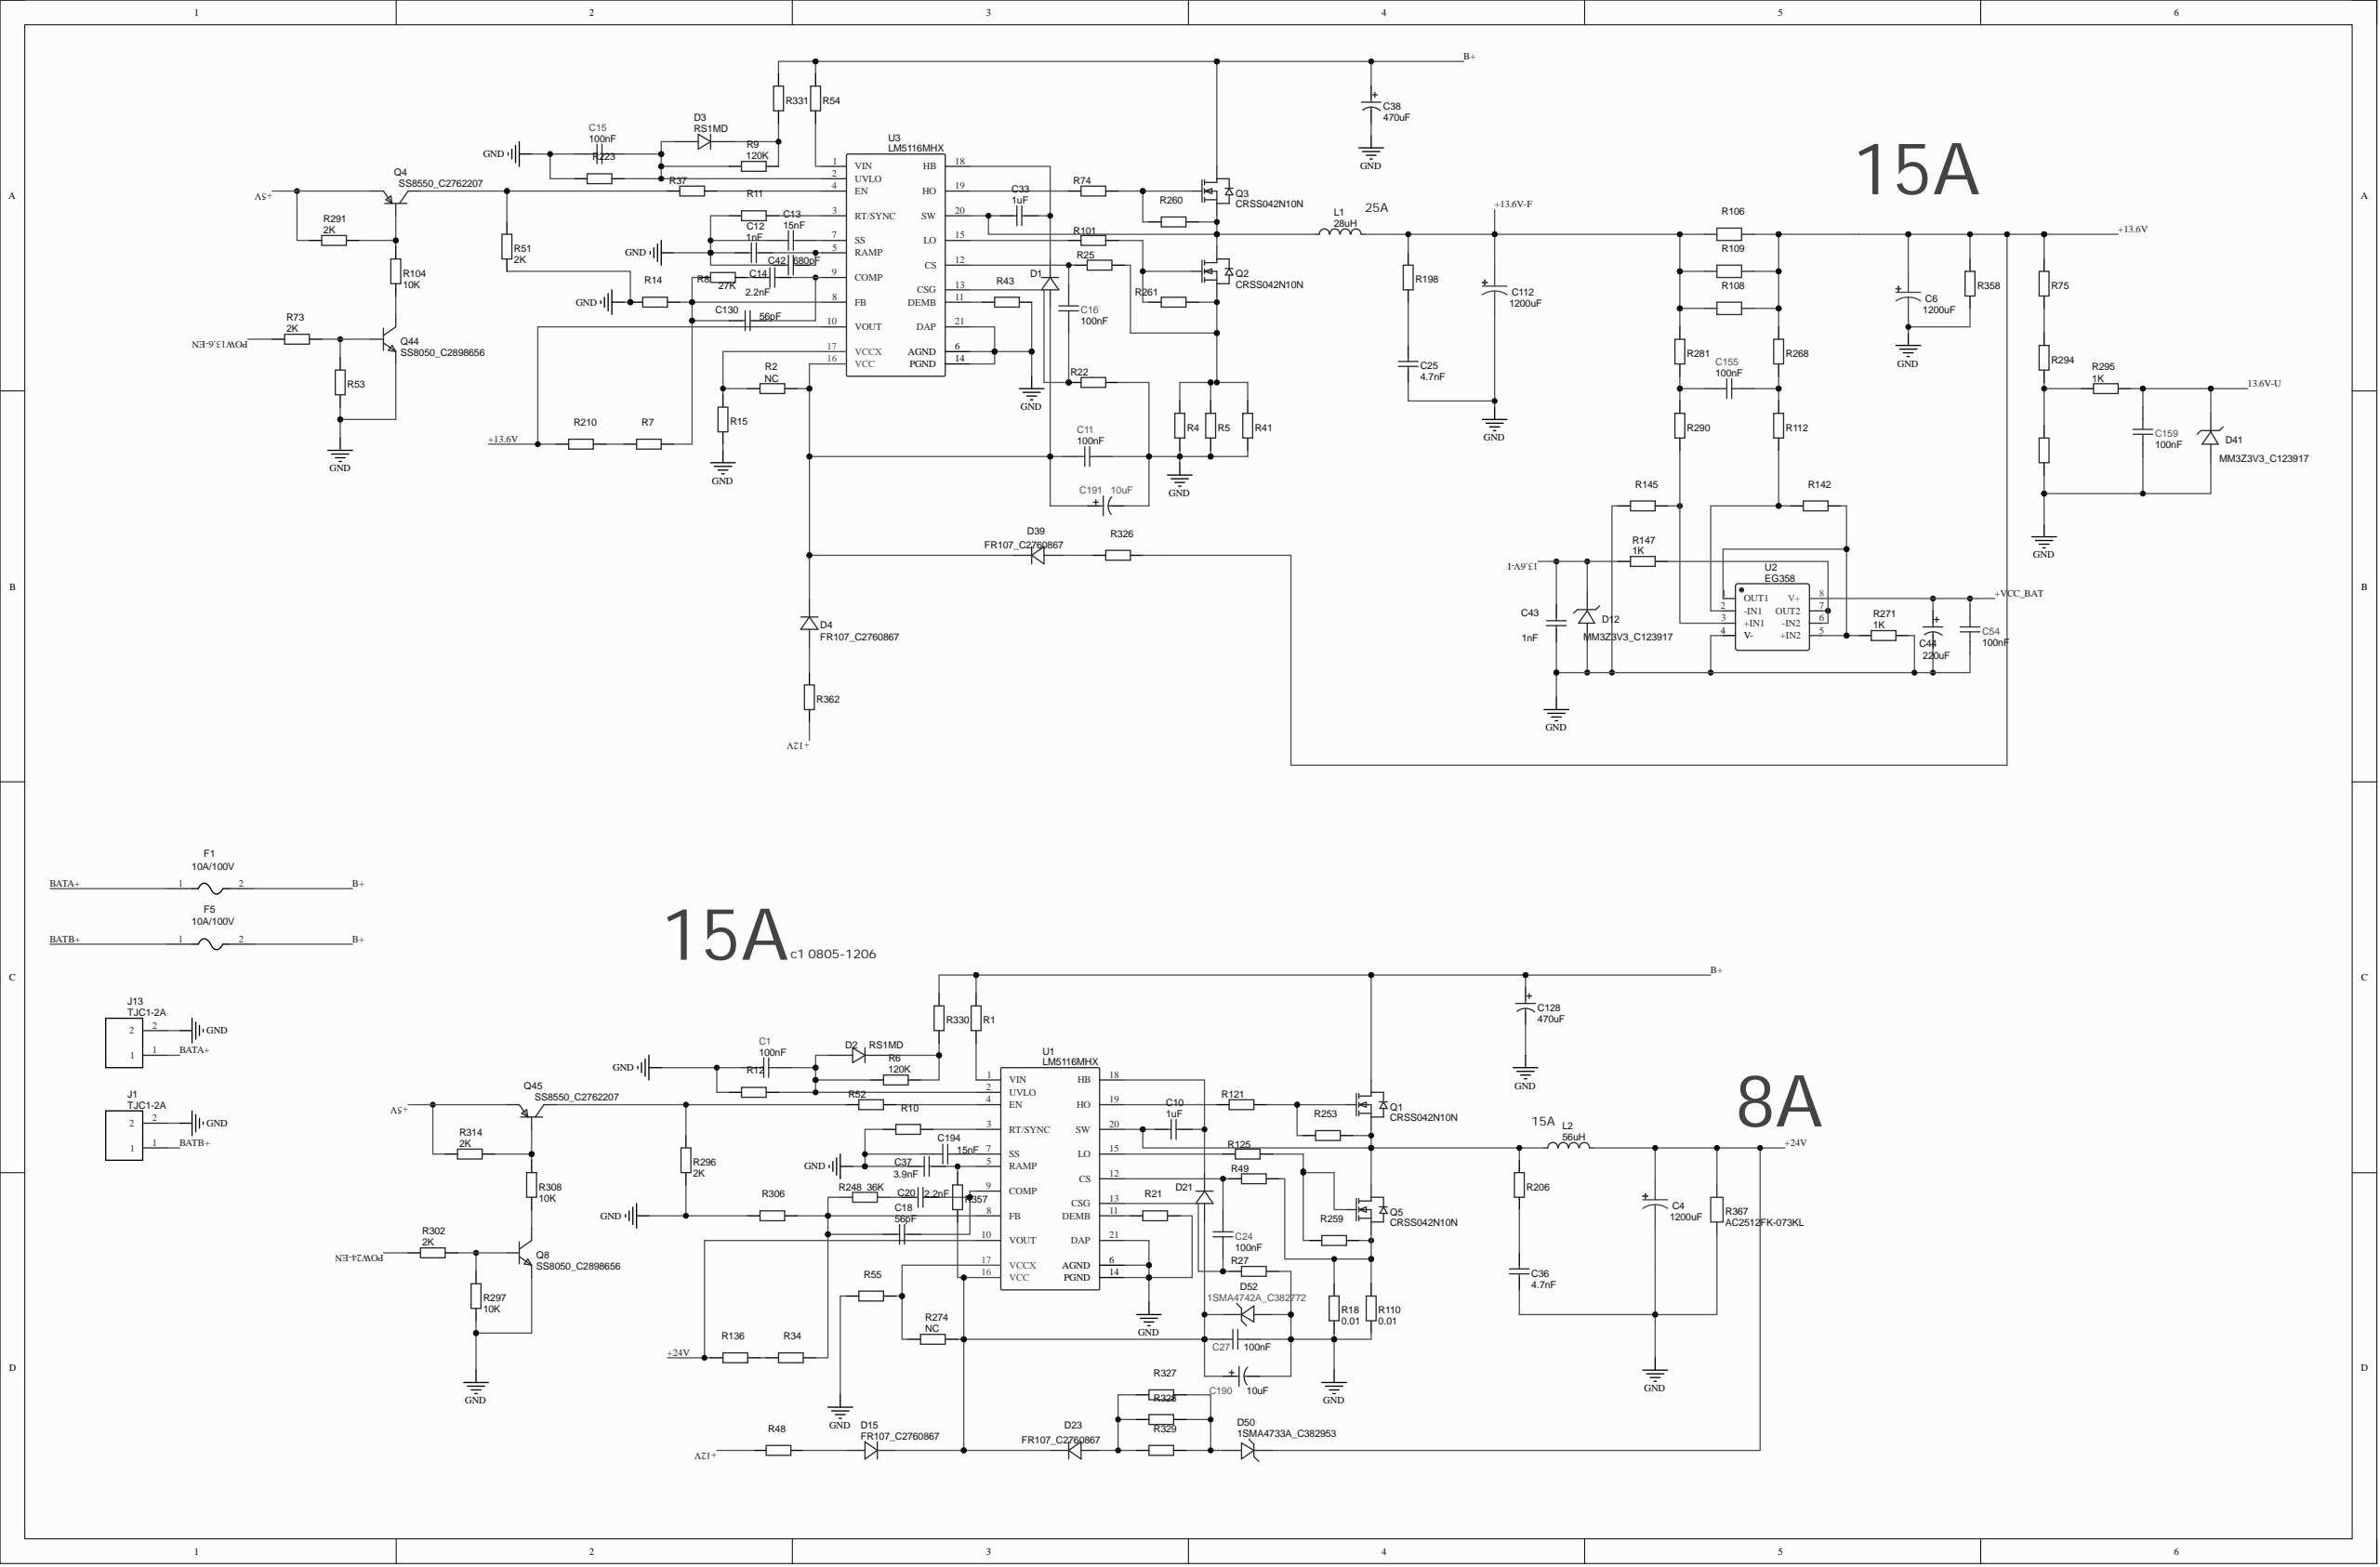Circuit board | Altium Designer | 694 parts | 423 nets | one sheet of the schematic
Parts on this sheet (reference | value | footprint):
C1 | 100nF | C0603
C4 | 1200uF | CAP-TH_BD13.0-P5.00-D1.2-FD
C6 | 1200uF | CAP-TH_BD13.0-P5.00-D1.2-FD
C10 | 1uF | C0603
C11 | 100nF | C0603
C12 | 1nF | C0603
C13 | 15nF | C0603
C14 | 2.2nF | C0603
C15 | 100nF | C0603
C16 | 100nF | C0603
C18 | 56pF | C0603
C20 | 2.2nF | C0603
C24 | 100nF | C0603
C25 | 4.7nF | C1206
C27 | 100nF | C0603
C33 | 1uF | C0603
C36 | 4.7nF | C1206
C37 | 3.9nF | C0603
C38 | 470uF | CAP-TH_BD12.5-P5.00-D0.6-FD
C42 | 680pF | C0603
C43 | 1nF | C0603
C44 | 220uF | CAP-TH_BD6.3-P2.50-D1.0-FD
C54 | 100nF | C0603
C112 | 1200uF | CAP-TH_BD13.0-P5.00-D1.2-FD
C128 | 470uF | CAP-TH_BD12.5-P5.00-D0.6-FD
C130 | 56pF | C0603
C155 | 100nF | C0603
C159 | 100nF | C0603
C190 | 10uF | CAP-TH_BD5.0-P2.5-D0.5-FD
C191 | 10uF | CAP-TH_BD5.0-P2.5-D0.5-FD
C194 | 15nF | C0603
D1 | FR107_C2760867 | SOD-123FL_L2.7-W1.8-LS3.8-RD
D2 | RS1MD | SMA_L4.3-W2.6-LS5.2-RD
D3 | RS1MD | SMA_L4.3-W2.6-LS5.2-RD
D4 | FR107_C2760867 | SOD-123FL_L2.7-W1.8-LS3.8-RD
D12 | MM3Z3V3_C123917 | SOD-323_L1.8-W1.3-LS2.5-RD
D15 | FR107_C2760867 | SOD-123FL_L2.7-W1.8-LS3.8-RD
D21 | FR107_C2760867 | SOD-123FL_L2.7-W1.8-LS3.8-RD
D23 | FR107_C2760867 | SOD-123FL_L2.7-W1.8-LS3.8-RD
D39 | FR107_C2760867 | SOD-123FL_L2.7-W1.8-LS3.8-RD
D41 | MM3Z3V3_C123917 | SOD-323_L1.8-W1.3-LS2.5-RD
D50 | 1SMA4733A_C382953 | SMA_L4.4-W2.6-LS5.0-RD
D52 | 1SMA4742A_C382772 | SMA_L4.4-W2.6-LS5.0-RD
F1 | 10A/100V | FUSE-SMD_L6.1-W2.5
F5 | 10A/100V | FUSE-SMD_L6.1-W2.5
J1 | TJC1-2A | CONN-TH_XT30UPB-F-W
J13 | TJC1-2A | CONN-TH_XT30UPB-F-W
L1 | 28uH | IND-TH_CS270026-W280M-N
L2 | 56uH | IND-TH_CS270026-W560M-N
Q1 | CRSS042N10N | TO-263-3_L10.2-W10.7-P5.08-LS16.2-TL
Q2 | CRSS042N10N | TO-263-3_L10.2-W10.7-P5.08-LS16.2-TL
Q3 | CRSS042N10N | TO-263-3_L10.2-W10.7-P5.08-LS16.2-TL
Q4 | SS8550_C2762207 | SOT-23-3_L2.9-W1.3-P1.90-LS2.4-BR
Q5 | CRSS042N10N | TO-263-3_L10.2-W10.7-P5.08-LS16.2-TL
Q8 | SS8050_C2898656 | SOT-23-3_L2.9-W1.3-P1.90-LS2.4-BR
Q44 | SS8050_C2898656 | SOT-23-3_L2.9-W1.3-P1.90-LS2.4-BR
Q45 | SS8550_C2762207 | SOT-23-3_L2.9-W1.3-P1.90-LS2.4-BR
R1 | R1206
R2 | NC | R0603
R4 | R2512
R5 | R2512
R6 | 120K | R0603
R7 | R0603
R8 | 27K | R0603
R9 | 120K | R0603
R10 | R0603
R11 | R0603
R12 | R0603
R14 | R0603
R15 | R0603
R18 | 0.01 | R2512
R21 | R0603
R22 | R0603
R25 | R0603
R27 | R0603
R34 | R0603
R37 | R0603
R41 | R2512
R43 | R0603
R48 | R0603
R49 | R0603
R51 | 2K | R0603
R52 | R0603
R53 | R0603
R54 | R1206
R55 | R0603
R73 | 2K | R0603
R74 | R0805
R75 | R0603
R101 | R0805
R104 | 10K | R0603
R106 | R2512
R108 | R2512
R109 | R2512
R110 | 0.01 | R2512
R112 | R0603
R121 | R0805
R125 | R0805
R136 | R0603
R142 | R0603
R145 | R0603
R147 | 1K | R0603
R198 | R1206
R206 | R1206
R210 | R0603
R223 | R0603
R248 | 36K | R0603
R253 | R0603
R259 | R0603
R260 | R0603
R261 | R0603
R268 | R0603
R271 | 1K | R0603
R274 | NC | R0603
R281 | R0603
R290 | R0603
R291 | 2K | R0603
R294 | R0603
R295 | 1K | R0603
R296 | 2K | R0603
R297 | 10K | R0603
R302 | 2K | R0603
R306 | R0603
R308 | 10K | R0603
R314 | 2K | R0603
R326 | R0603
R327 | R0805
R328 | R0805
R329 | R0805
R330 | R1206
R331 | R1206
R357 | R0603
R358 | R2512
R362 | R0603
R367 | AC2512FK-073KL | R2512
U1 | LM5116MHX | HTSSOP-20_L6.5-W4.4-P0.65-LS6.4-BL-EP
U2 | EG358 | SOIC-8_L5.0-W4.0-P1.27-LS6.0-BL
U3 | LM5116MHX | HTSSOP-20_L6.5-W4.4-P0.65-LS6.4-BL-EP
Nets of these parts (net: part-pin ...):
POW24-EN: R302-1
POW13.6-EN: R73-1
NetR147_1: R147-1 U2-6 U2-7
NetR145_2: R145-2 R290-2 U2-3
NetR142_2: R142-2 R271-1 U2-1 U2-5
NetR125_2: R125-2 U1-15
NetR121_2: R121-2 U1-19
NetR112_2: R112-2 R142-1 U2-2
NetR107_2: R294-1 R295-2
NetR101_2: R101-2 U3-15
NetR75_1: R75-1 R294-2
NetR74_2: R74-2 U3-19
NetR55_2: R55-2 R274-1 U1-17
NetR54_1: R54-1 U3-1
NetR52_2: R52-2 U1-4
NetR43_1: R43-1 U3-11
NetR37_2: R37-2 U3-4
NetR34_1: R34-1 R136-1
NetR21_1: R21-1 U1-11
NetR11_2: R11-2 U3-3
NetR10_2: R10-2 U1-3
NetR7_1: R7-1 R210-2
NetR2_1: R2-1 R15-2 U3-17
NetR1_1: R1-1 U1-1
NetQ45_3: Q45-3 R52-1 R296-2
NetQ45_1: Q45-1 R308-2 R314-2
NetQ44_3: Q44-3 R104-1
NetQ44_1: Q44-1 R53-1 R73-2
NetQ8_3: Q8-3 R308-1
NetQ8_1: Q8-1 R297-1 R302-2
NetQ5_3: Q5-3 R18-2 R49-1 R110-2 R259-1
NetQ5_1: Q5-1 R125-1 R259-2
NetQ4_3: Q4-3 R37-1 R51-2
NetQ4_1: Q4-1 R104-2 R291-2
NetQ3_1: Q3-1 R74-1 R260-2
NetQ2_3: Q2-3 R4-2 R5-2 R25-1 R41-2 R261-1
NetQ2_1: Q2-1 R101-1 R261-2
NetQ1_1: Q1-1 R121-1 R253-2
NetD50_2: D50-2 R327-2 R328-2 R329-2
NetD39_2: D39-2 R326-1
NetD23_2: D23-2 R327-1 R328-1 R329-1
NetD15_2: D15-2 R48-1
NetD4_2: D4-2 R362-2
NetD3_1: D3-1 R9-2 R331-1
NetD2_1: D2-1 R6-2 R330-1
NetC194_1: C194-1 U1-7
NetC155_2: C155-2 R281-2 R290-1
NetC155_1: C155-1 R112-1 R268-2
NetC130_2: C130-2 R7-2 R8-1 R14-1 U3-8
NetC37_1: C37-1 R357-2 U1-5
NetC36_2: C36-2 R206-1
NetC33_2: C33-2 D1-1 U3-18
NetC33_1: C33-1 L1-1 Q2-2 Q3-3 R260-1 U3-20
NetC27_2: C27-2 C190-1 D15-1 D21-2 D23-1 D52-1 R274-2 R357-1 U1-16
NetC25_2: C25-2 R198-1
NetC24_2: C24-2 R27-2 U1-13
NetC24_1: C24-1 R49-2 U1-12
NetC20_2: C20-2 R248-2
NetC18_2: C18-2 R34-2 R248-1 R306-1 U1-8
NetC18_1: C18-1 C20-1 U1-9
NetC16_2: C16-2 R22-2 U3-13
NetC16_1: C16-1 R25-2 U3-12
NetC15_1: C15-1 D3-2 R9-1 R223-2 U3-2
NetC14_2: C14-2 C130-1 U3-9
NetC14_1: C14-1 R8-2
NetC13_1: C13-1 U3-7
NetC12_2: C12-2 C42-2 U3-5
NetC11_2: C11-2 C191-1 D1-2 D4-1 D39-1 R2-2 U3-16
NetC10_2: C10-2 D21-1 U1-18
NetC10_1: C10-1 L2-1 Q1-3 Q5-2 R206-2 R253-1 U1-20
NetC1_1: C1-1 D2-2 R6-1 R12-2 U1-2
GND: C1-2 C4-2 C6-2 C11-1 C12-1 C13-2 C15-2 C25-1 C27-1 C36-1 C37-2 C38-2 C42-1 C43-1 C44-2 C54-2 C112-2 C128-2 C159-2 C190-2 C191-2 C194-2 D12-2 D41-2 D52-2 J1-2 J13-2 Q8-2 Q44-2 R4-1 R5-1 R10-1 R11-1 R12-1 R14-2 R15-1 R18-1 R21-2 R22-1 R27-1 R41-1 R43-2 R51-1 R53-2 R55-1 R110-1 R145-1 R223-1 R271-2 R296-1 R297-2 R306-2 R358-1 R367-1 U2-4 U1-6 U1-14 U1-21 U3-6 U3-14 U3-21
BATB+: F5-1 J1-1
BATA+: F1-1 J13-1
B+: C38-1 C128-1 F1-2 F5-2 Q1-2 Q3-2 R1-2 R54-2 R330-2 R331-2
+VCC_BAT: C44-1 C54-1 U2-8
+24V: C4-1 D50-1 L2-2 R136-2 R367-2 U1-10
+13.6V-F: C112-1 L1-2 R106-1 R108-1 R109-1 R198-2 R281-1
+13.6V: C6-1 R75-2 R106-2 R108-2 R109-2 R210-1 R268-1 R326-2 R358-2 U3-10
+12V: R48-2 R362-1
+5V: Q4-2 Q45-2 R291-1 R314-1
13.6V-U: C159-1 D41-1 R295-1
13.6V-I: C43-2 D12-1 R147-2